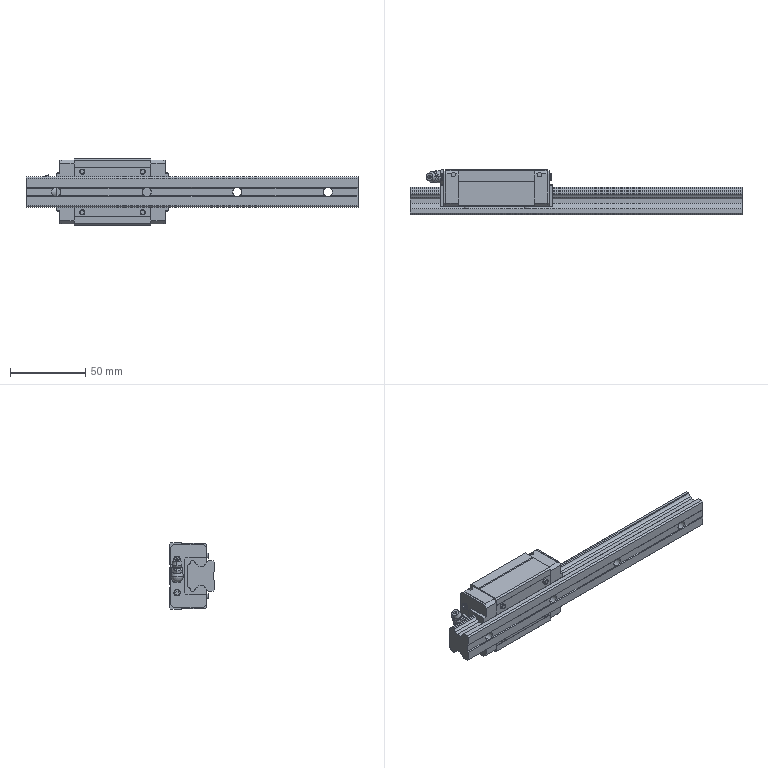Part | SolidWorks | 3 solids | 356 faces | box 220 x 30 x 44 mm | volume 122674 mm3 | plane 208 | cylinder 84 | cone 36 | torus 22 | sphere 6 | commonest cylinder face diameters 4.134 x16 6 x14 3 x8 3.43 x8 4.12 x8 4.5 x8